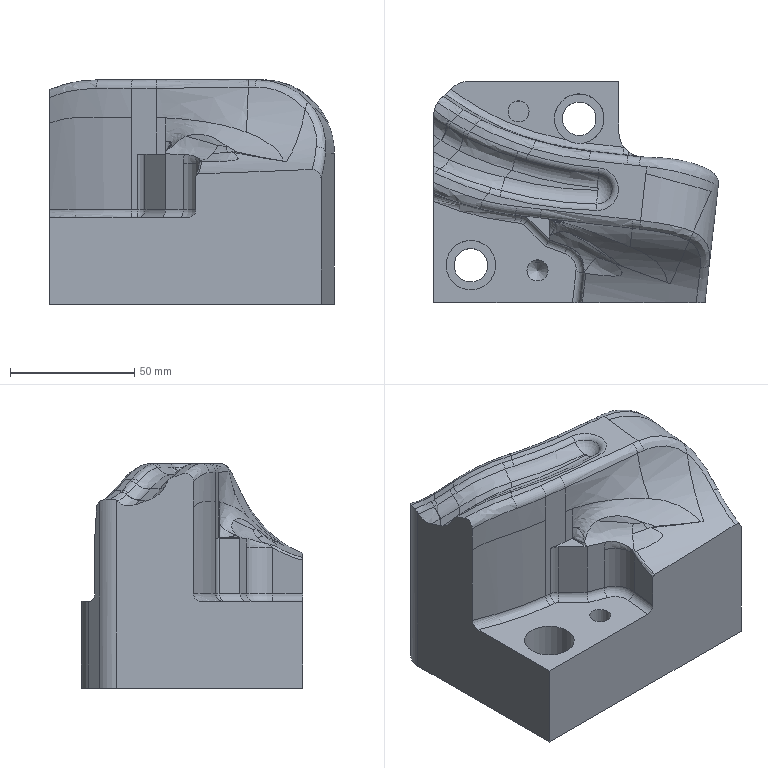Part | NX | features 23 2 | 1 solid | 127 faces | box 114.705 x 89 x 90.4 mm | volume 512354 mm3 | spline 44 | plane 36 | cylinder 34 | torus 12 | cone 1 | commonest cylinder face diameters 20 x6 6 x4 7 x4 15 x4 8.5 x2 13.5 x2